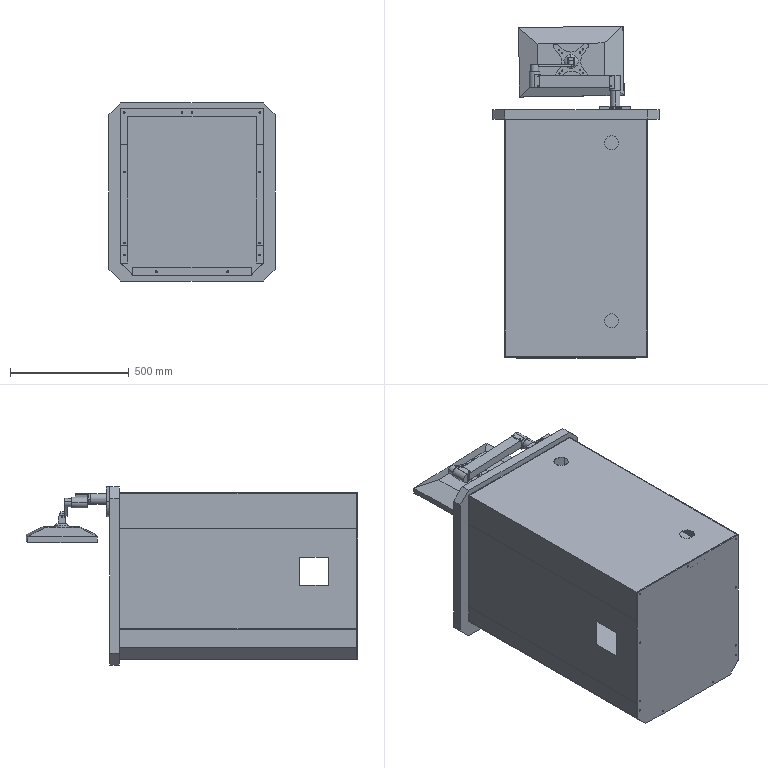Part | SolidWorks | features AEMSimFeature 1 | 15 solids | 456 faces | box 700 x 1398 x 750 mm | volume 37335831 mm3 | cylinder 239 | plane 215 | spline 2 | commonest cylinder face diameters 6 x130 5 x66 20 x10 10 x6 45 x6 60 x6